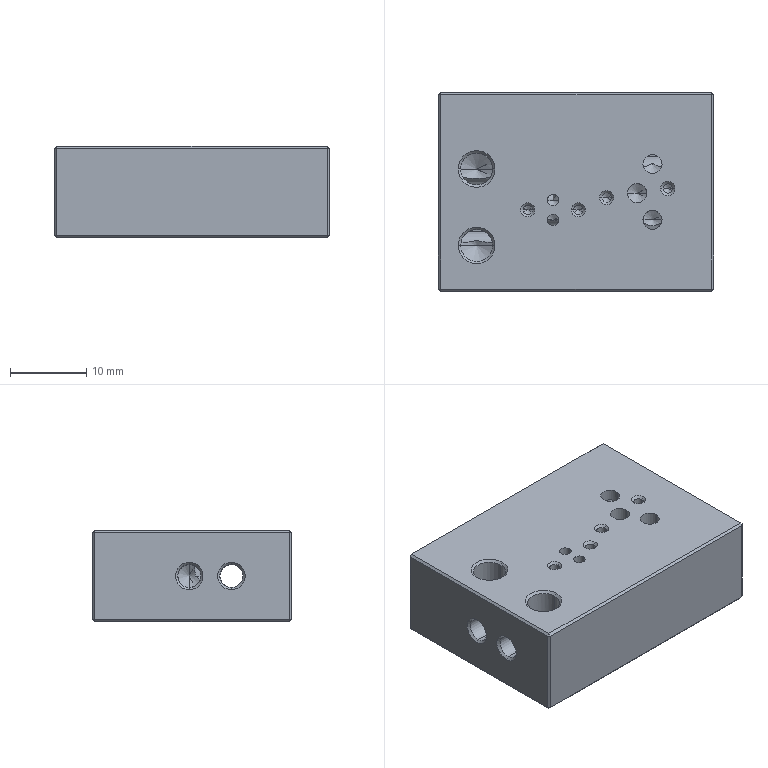Part | SolidWorks | features HoleWzd 14, MoveCopyBody 7, Stock 7, Chamfer 1, Extrusion 1, MoveFace 1 | 1 solid | 142 faces | box 36 x 26 x 12 mm | volume 10025 mm3 | cone 70 | cylinder 46 | plane 26 | commonest cylinder face diameters 2.5 x16 3 x10 1.25 x8 4.2 x8 1.5 x4